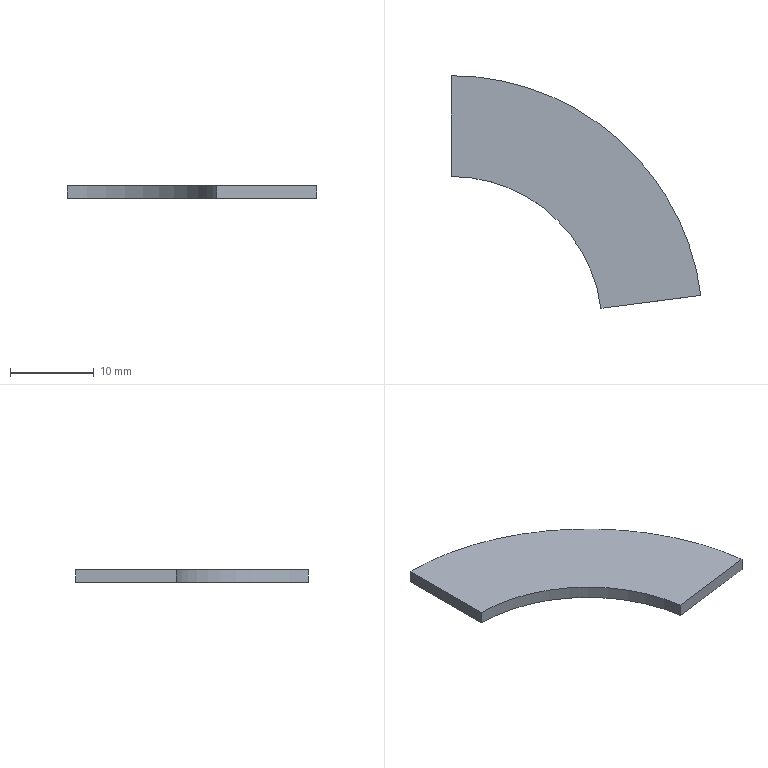Part | STEP file | FHD-021-012-D side door A-D | 1 solid | 6 faces | box 29.753 x 27.697 x 1.5 mm | volume 623.148 mm3 | plane 4 | cylinder 2 | commonest cylinder face diameters 36 x1 60 x1
STEP:
#1=CARTESIAN_POINT('',(0.,0.,0.));
#2=DIRECTION('',(0.,0.,1.));
#3=DIRECTION('',(1.,0.,0.));
#4=AXIS2_PLACEMENT_3D('',#1,#2,#3);
#5=CARTESIAN_POINT('',(1852.179,1263.266,-1.5));
#6=VERTEX_POINT('',#5);
#7=CARTESIAN_POINT('',(1864.08,1264.802,-1.5));
#8=VERTEX_POINT('',#7);
#9=CARTESIAN_POINT('',(1852.179,1263.266,-1.5));
#10=DIRECTION('',(0.9918,0.128,0.));
#11=VECTOR('',#10,1.);
#12=LINE('',#9,#11);
#13=CARTESIAN_POINT('',(1834.327,1260.963,-1.5));
#14=DIRECTION('',(0.,0.,1.));
#15=DIRECTION('',(1.,0.,0.));
#16=AXIS2_PLACEMENT_3D('',#13,#14,#15);
#17=PLANE('',#16);
#18=CARTESIAN_POINT('',(17.852,2.303));
#19=DIRECTION('',(0.9918,0.128));
#20=VECTOR('',#19,1.);
#21=LINE('',#18,#20);
#22=(GEOMETRIC_REPRESENTATION_CONTEXT(2)PARAMETRIC_REPRESENTATION_CONTEXT()REPRESENTATION_CONTEXT('',''));
#23=DEFINITIONAL_REPRESENTATION('',(#21),#22);
#24=PCURVE('',#17,#23);
#25=CARTESIAN_POINT('',(1852.179,1263.266,-1.5));
#26=DIRECTION('',(0.128,-0.9918,0.));
#27=DIRECTION('',(0.9918,0.128,0.));
#28=AXIS2_PLACEMENT_3D('',#25,#26,#27);
#29=PLANE('',#28);
#30=CARTESIAN_POINT('',(0.,0.));
#31=DIRECTION('',(1.,0.));
#32=VECTOR('',#31,1.);
#33=LINE('',#30,#32);
#34=(GEOMETRIC_REPRESENTATION_CONTEXT(2)PARAMETRIC_REPRESENTATION_CONTEXT()REPRESENTATION_CONTEXT('',''));
#35=DEFINITIONAL_REPRESENTATION('',(#33),#34);
#36=PCURVE('',#29,#35);
#37=SURFACE_CURVE('',#12,(#24,#36),.PCURVE_S1.);
#38=EDGE_CURVE('',#6,#8,#37,.T.);
#39=ORIENTED_EDGE('',*,*,#38,.F.);
#40=CARTESIAN_POINT('',(1834.327,1278.963,-1.5));
#41=VERTEX_POINT('',#40);
#42=CARTESIAN_POINT('',(1834.327,1260.963,-1.5));
#43=DIRECTION('',(0.,0.,-1.));
#44=DIRECTION('',(1.,0.,0.));
#45=AXIS2_PLACEMENT_3D('',#42,#43,#44);
#46=CIRCLE('',#45,18.);
#47=CARTESIAN_POINT('',(18.,0.));
#48=CARTESIAN_POINT('',(18.,-31.177));
#49=CARTESIAN_POINT('',(-9.,-15.588));
#50=CARTESIAN_POINT('',(-36.,0.));
#51=CARTESIAN_POINT('',(-9.,15.588));
#52=CARTESIAN_POINT('',(18.,31.177));
#53=CARTESIAN_POINT('',(18.,0.));
#54=(BOUNDED_CURVE()B_SPLINE_CURVE(2,(#47,#48,#49,#50,#51,#52,#53),.UNSPECIFIED.,.T.,.F.)B_SPLINE_CURVE_WITH_KNOTS((1,2,2,2,2,1),(-2.094,0.,2.094,4.189,6.283,8.378),.UNSPECIFIED.)CURVE()GEOMETRIC_REPRESENTATION_ITEM()RATIONAL_B_SPLINE_CURVE((1.,0.5,1.,0.5,1.,0.5,1.))REPRESENTATION_ITEM(''));
#55=(GEOMETRIC_REPRESENTATION_CONTEXT(2)PARAMETRIC_REPRESENTATION_CONTEXT()REPRESENTATION_CONTEXT('',''));
#56=DEFINITIONAL_REPRESENTATION('',(#54),#55);
#57=PCURVE('',#17,#56);
#58=CARTESIAN_POINT('',(1834.327,1260.963,-1.5));
#59=DIRECTION('',(0.,0.,1.));
#60=DIRECTION('',(1.,0.,0.));
#61=AXIS2_PLACEMENT_3D('',#58,#59,#60);
#62=CYLINDRICAL_SURFACE('',#61,18.);
#63=CARTESIAN_POINT('',(6.283,0.));
#64=DIRECTION('',(-1.,0.));
#65=VECTOR('',#64,1.);
#66=LINE('',#63,#65);
#67=(GEOMETRIC_REPRESENTATION_CONTEXT(2)PARAMETRIC_REPRESENTATION_CONTEXT()REPRESENTATION_CONTEXT('',''));
#68=DEFINITIONAL_REPRESENTATION('',(#66),#67);
#69=PCURVE('',#62,#68);
#70=SURFACE_CURVE('',#46,(#57,#69),.PCURVE_S1.);
#71=EDGE_CURVE('',#41,#6,#70,.T.);
#72=ORIENTED_EDGE('',*,*,#71,.F.);
#73=CARTESIAN_POINT('',(1834.327,1290.963,-1.5));
#74=VERTEX_POINT('',#73);
#75=CARTESIAN_POINT('',(1834.327,1260.963,-1.5));
#76=DIRECTION('',(0.,-1.,0.));
#77=VECTOR('',#76,1.);
#78=LINE('',#75,#77);
#79=CARTESIAN_POINT('',(0.,0.));
#80=DIRECTION('',(0.,-1.));
#81=VECTOR('',#80,1.);
#82=LINE('',#79,#81);
#83=(GEOMETRIC_REPRESENTATION_CONTEXT(2)PARAMETRIC_REPRESENTATION_CONTEXT()REPRESENTATION_CONTEXT('',''));
#84=DEFINITIONAL_REPRESENTATION('',(#82),#83);
#85=PCURVE('',#17,#84);
#86=CARTESIAN_POINT('',(1834.327,1290.963,-1.5));
#87=DIRECTION('',(-1.,0.,0.));
#88=DIRECTION('',(0.,0.,1.));
#89=AXIS2_PLACEMENT_3D('',#86,#87,#88);
#90=PLANE('',#89);
#91=CARTESIAN_POINT('',(0.,-30.));
#92=DIRECTION('',(0.,-1.));
#93=VECTOR('',#92,1.);
#94=LINE('',#91,#93);
#95=(GEOMETRIC_REPRESENTATION_CONTEXT(2)PARAMETRIC_REPRESENTATION_CONTEXT()REPRESENTATION_CONTEXT('',''));
#96=DEFINITIONAL_REPRESENTATION('',(#94),#95);
#97=PCURVE('',#90,#96);
#98=SURFACE_CURVE('',#78,(#85,#97),.PCURVE_S1.);
#99=EDGE_CURVE('',#74,#41,#98,.T.);
#100=ORIENTED_EDGE('',*,*,#99,.F.);
#101=CARTESIAN_POINT('',(1834.327,1260.963,-1.5));
#102=DIRECTION('',(0.,0.,1.));
#103=DIRECTION('',(1.,0.,0.));
#104=AXIS2_PLACEMENT_3D('',#101,#102,#103);
#105=CIRCLE('',#104,30.);
#106=CARTESIAN_POINT('',(0.,0.));
#107=DIRECTION('',(1.,0.));
#108=AXIS2_PLACEMENT_2D('',#106,#107);
#109=CIRCLE('',#108,30.);
#110=(GEOMETRIC_REPRESENTATION_CONTEXT(2)PARAMETRIC_REPRESENTATION_CONTEXT()REPRESENTATION_CONTEXT('',''));
#111=DEFINITIONAL_REPRESENTATION('',(#109),#110);
#112=PCURVE('',#17,#111);
#113=CARTESIAN_POINT('',(1834.327,1260.963,-1.5));
#114=DIRECTION('',(0.,0.,1.));
#115=DIRECTION('',(1.,0.,0.));
#116=AXIS2_PLACEMENT_3D('',#113,#114,#115);
#117=CYLINDRICAL_SURFACE('',#116,30.);
#118=CARTESIAN_POINT('',(0.,0.));
#119=DIRECTION('',(1.,0.));
#120=VECTOR('',#119,1.);
#121=LINE('',#118,#120);
#122=(GEOMETRIC_REPRESENTATION_CONTEXT(2)PARAMETRIC_REPRESENTATION_CONTEXT()REPRESENTATION_CONTEXT('',''));
#123=DEFINITIONAL_REPRESENTATION('',(#121),#122);
#124=PCURVE('',#117,#123);
#125=SURFACE_CURVE('',#105,(#112,#124),.PCURVE_S1.);
#126=EDGE_CURVE('',#8,#74,#125,.T.);
#127=ORIENTED_EDGE('',*,*,#126,.F.);
#128=EDGE_LOOP('',(#39,#72,#100,#127));
#129=FACE_BOUND('',#128,.T.);
#130=ADVANCED_FACE('',(#129),#17,.F.);
#131=ORIENTED_EDGE('',*,*,#126,.T.);
#132=CARTESIAN_POINT('',(1834.327,1290.963,0.));
#133=VERTEX_POINT('',#132);
#134=CARTESIAN_POINT('',(1834.327,1290.963,-1.5));
#135=DIRECTION('',(0.,0.,1.));
#136=VECTOR('',#135,1.);
#137=LINE('',#134,#136);
#138=CARTESIAN_POINT('',(1.571,0.));
#139=DIRECTION('',(0.,1.));
#140=VECTOR('',#139,1.);
#141=LINE('',#138,#140);
#142=(GEOMETRIC_REPRESENTATION_CONTEXT(2)PARAMETRIC_REPRESENTATION_CONTEXT()REPRESENTATION_CONTEXT('',''));
#143=DEFINITIONAL_REPRESENTATION('',(#141),#142);
#144=PCURVE('',#117,#143);
#145=CARTESIAN_POINT('',(0.,0.));
#146=DIRECTION('',(1.,0.));
#147=VECTOR('',#146,1.);
#148=LINE('',#145,#147);
#149=(GEOMETRIC_REPRESENTATION_CONTEXT(2)PARAMETRIC_REPRESENTATION_CONTEXT()REPRESENTATION_CONTEXT('',''));
#150=DEFINITIONAL_REPRESENTATION('',(#148),#149);
#151=PCURVE('',#90,#150);
#152=SURFACE_CURVE('',#137,(#144,#151),.PCURVE_S1.);
#153=EDGE_CURVE('',#74,#133,#152,.T.);
#154=ORIENTED_EDGE('',*,*,#153,.T.);
#155=CARTESIAN_POINT('',(1864.08,1264.802,0.));
#156=VERTEX_POINT('',#155);
#157=CARTESIAN_POINT('',(1834.327,1260.963,0.));
#158=DIRECTION('',(0.,0.,-1.));
#159=DIRECTION('',(1.,0.,0.));
#160=AXIS2_PLACEMENT_3D('',#157,#158,#159);
#161=CIRCLE('',#160,30.);
#162=CARTESIAN_POINT('',(6.283,1.5));
#163=DIRECTION('',(-1.,0.));
#164=VECTOR('',#163,1.);
#165=LINE('',#162,#164);
#166=(GEOMETRIC_REPRESENTATION_CONTEXT(2)PARAMETRIC_REPRESENTATION_CONTEXT()REPRESENTATION_CONTEXT('',''));
#167=DEFINITIONAL_REPRESENTATION('',(#165),#166);
#168=PCURVE('',#117,#167);
#169=CARTESIAN_POINT('',(1834.327,1260.963,0.));
#170=DIRECTION('',(0.,0.,1.));
#171=DIRECTION('',(1.,0.,0.));
#172=AXIS2_PLACEMENT_3D('',#169,#170,#171);
#173=PLANE('',#172);
#174=CARTESIAN_POINT('',(30.,0.));
#175=CARTESIAN_POINT('',(30.,-51.962));
#176=CARTESIAN_POINT('',(-15.,-25.981));
#177=CARTESIAN_POINT('',(-60.,0.));
#178=CARTESIAN_POINT('',(-15.,25.981));
#179=CARTESIAN_POINT('',(30.,51.962));
#180=CARTESIAN_POINT('',(30.,0.));
#181=(BOUNDED_CURVE()B_SPLINE_CURVE(2,(#174,#175,#176,#177,#178,#179,#180),.UNSPECIFIED.,.T.,.F.)B_SPLINE_CURVE_WITH_KNOTS((1,2,2,2,2,1),(-2.094,0.,2.094,4.189,6.283,8.378),.UNSPECIFIED.)CURVE()GEOMETRIC_REPRESENTATION_ITEM()RATIONAL_B_SPLINE_CURVE((1.,0.5,1.,0.5,1.,0.5,1.))REPRESENTATION_ITEM(''));
#182=(GEOMETRIC_REPRESENTATION_CONTEXT(2)PARAMETRIC_REPRESENTATION_CONTEXT()REPRESENTATION_CONTEXT('',''));
#183=DEFINITIONAL_REPRESENTATION('',(#181),#182);
#184=PCURVE('',#173,#183);
#185=SURFACE_CURVE('',#161,(#168,#184),.PCURVE_S1.);
#186=EDGE_CURVE('',#133,#156,#185,.T.);
#187=ORIENTED_EDGE('',*,*,#186,.T.);
#188=CARTESIAN_POINT('',(1864.08,1264.802,-1.5));
#189=DIRECTION('',(0.,0.,-1.));
#190=VECTOR('',#189,1.);
#191=LINE('',#188,#190);
#192=CARTESIAN_POINT('',(0.1283,0.));
#193=DIRECTION('',(0.,-1.));
#194=VECTOR('',#193,1.);
#195=LINE('',#192,#194);
#196=(GEOMETRIC_REPRESENTATION_CONTEXT(2)PARAMETRIC_REPRESENTATION_CONTEXT()REPRESENTATION_CONTEXT('',''));
#197=DEFINITIONAL_REPRESENTATION('',(#195),#196);
#198=PCURVE('',#117,#197);
#199=CARTESIAN_POINT('',(12.,0.));
#200=DIRECTION('',(0.,-1.));
#201=VECTOR('',#200,1.);
#202=LINE('',#199,#201);
#203=(GEOMETRIC_REPRESENTATION_CONTEXT(2)PARAMETRIC_REPRESENTATION_CONTEXT()REPRESENTATION_CONTEXT('',''));
#204=DEFINITIONAL_REPRESENTATION('',(#202),#203);
#205=PCURVE('',#29,#204);
#206=SURFACE_CURVE('',#191,(#198,#205),.PCURVE_S1.);
#207=EDGE_CURVE('',#156,#8,#206,.T.);
#208=ORIENTED_EDGE('',*,*,#207,.T.);
#209=EDGE_LOOP('',(#131,#154,#187,#208));
#210=FACE_BOUND('',#209,.T.);
#211=ADVANCED_FACE('',(#210),#117,.T.);
#212=ORIENTED_EDGE('',*,*,#38,.T.);
#213=ORIENTED_EDGE('',*,*,#207,.F.);
#214=CARTESIAN_POINT('',(1852.179,1263.266,0.));
#215=VERTEX_POINT('',#214);
#216=CARTESIAN_POINT('',(1852.179,1263.266,0.));
#217=DIRECTION('',(-0.9918,-0.128,0.));
#218=VECTOR('',#217,1.);
#219=LINE('',#216,#218);
#220=CARTESIAN_POINT('',(0.,1.5));
#221=DIRECTION('',(-1.,0.));
#222=VECTOR('',#221,1.);
#223=LINE('',#220,#222);
#224=(GEOMETRIC_REPRESENTATION_CONTEXT(2)PARAMETRIC_REPRESENTATION_CONTEXT()REPRESENTATION_CONTEXT('',''));
#225=DEFINITIONAL_REPRESENTATION('',(#223),#224);
#226=PCURVE('',#29,#225);
#227=CARTESIAN_POINT('',(17.852,2.303));
#228=DIRECTION('',(-0.9918,-0.128));
#229=VECTOR('',#228,1.);
#230=LINE('',#227,#229);
#231=(GEOMETRIC_REPRESENTATION_CONTEXT(2)PARAMETRIC_REPRESENTATION_CONTEXT()REPRESENTATION_CONTEXT('',''));
#232=DEFINITIONAL_REPRESENTATION('',(#230),#231);
#233=PCURVE('',#173,#232);
#234=SURFACE_CURVE('',#219,(#226,#233),.PCURVE_S1.);
#235=EDGE_CURVE('',#156,#215,#234,.T.);
#236=ORIENTED_EDGE('',*,*,#235,.T.);
#237=CARTESIAN_POINT('',(1852.179,1263.266,-1.5));
#238=DIRECTION('',(0.,0.,-1.));
#239=VECTOR('',#238,1.);
#240=LINE('',#237,#239);
#241=CARTESIAN_POINT('',(0.,0.));
#242=DIRECTION('',(0.,-1.));
#243=VECTOR('',#242,1.);
#244=LINE('',#241,#243);
#245=(GEOMETRIC_REPRESENTATION_CONTEXT(2)PARAMETRIC_REPRESENTATION_CONTEXT()REPRESENTATION_CONTEXT('',''));
#246=DEFINITIONAL_REPRESENTATION('',(#244),#245);
#247=PCURVE('',#29,#246);
#248=CARTESIAN_POINT('',(0.1283,0.));
#249=DIRECTION('',(0.,-1.));
#250=VECTOR('',#249,1.);
#251=LINE('',#248,#250);
#252=(GEOMETRIC_REPRESENTATION_CONTEXT(2)PARAMETRIC_REPRESENTATION_CONTEXT()REPRESENTATION_CONTEXT('',''));
#253=DEFINITIONAL_REPRESENTATION('',(#251),#252);
#254=PCURVE('',#62,#253);
#255=SURFACE_CURVE('',#240,(#247,#254),.PCURVE_S1.);
#256=EDGE_CURVE('',#215,#6,#255,.T.);
#257=ORIENTED_EDGE('',*,*,#256,.T.);
#258=EDGE_LOOP('',(#212,#213,#236,#257));
#259=FACE_BOUND('',#258,.T.);
#260=ADVANCED_FACE('',(#259),#29,.T.);
#261=CARTESIAN_POINT('',(1834.327,1278.963,0.));
#262=VERTEX_POINT('',#261);
#263=CARTESIAN_POINT('',(1834.327,1260.963,0.));
#264=DIRECTION('',(0.,0.,-1.));
#265=DIRECTION('',(1.,0.,0.));
#266=AXIS2_PLACEMENT_3D('',#263,#264,#265);
#267=CIRCLE('',#266,18.);
#268=CARTESIAN_POINT('',(6.283,1.5));
#269=DIRECTION('',(-1.,0.));
#270=VECTOR('',#269,1.);
#271=LINE('',#268,#270);
#272=(GEOMETRIC_REPRESENTATION_CONTEXT(2)PARAMETRIC_REPRESENTATION_CONTEXT()REPRESENTATION_CONTEXT('',''));
#273=DEFINITIONAL_REPRESENTATION('',(#271),#272);
#274=PCURVE('',#62,#273);
#275=CARTESIAN_POINT('',(18.,0.));
#276=CARTESIAN_POINT('',(18.,-31.177));
#277=CARTESIAN_POINT('',(-9.,-15.588));
#278=CARTESIAN_POINT('',(-36.,0.));
#279=CARTESIAN_POINT('',(-9.,15.588));
#280=CARTESIAN_POINT('',(18.,31.177));
#281=CARTESIAN_POINT('',(18.,0.));
#282=(BOUNDED_CURVE()B_SPLINE_CURVE(2,(#275,#276,#277,#278,#279,#280,#281),.UNSPECIFIED.,.T.,.F.)B_SPLINE_CURVE_WITH_KNOTS((1,2,2,2,2,1),(-2.094,0.,2.094,4.189,6.283,8.378),.UNSPECIFIED.)CURVE()GEOMETRIC_REPRESENTATION_ITEM()RATIONAL_B_SPLINE_CURVE((1.,0.5,1.,0.5,1.,0.5,1.))REPRESENTATION_ITEM(''));
#283=(GEOMETRIC_REPRESENTATION_CONTEXT(2)PARAMETRIC_REPRESENTATION_CONTEXT()REPRESENTATION_CONTEXT('',''));
#284=DEFINITIONAL_REPRESENTATION('',(#282),#283);
#285=PCURVE('',#173,#284);
#286=SURFACE_CURVE('',#267,(#274,#285),.PCURVE_S1.);
#287=EDGE_CURVE('',#262,#215,#286,.T.);
#288=ORIENTED_EDGE('',*,*,#287,.T.);
#289=ORIENTED_EDGE('',*,*,#256,.T.);
#290=ORIENTED_EDGE('',*,*,#71,.F.);
#291=CARTESIAN_POINT('',(1834.327,1278.963,-1.5));
#292=DIRECTION('',(0.,0.,1.));
#293=VECTOR('',#292,1.);
#294=LINE('',#291,#293);
#295=CARTESIAN_POINT('',(1.571,0.));
#296=DIRECTION('',(0.,1.));
#297=VECTOR('',#296,1.);
#298=LINE('',#295,#297);
#299=(GEOMETRIC_REPRESENTATION_CONTEXT(2)PARAMETRIC_REPRESENTATION_CONTEXT()REPRESENTATION_CONTEXT('',''));
#300=DEFINITIONAL_REPRESENTATION('',(#298),#299);
#301=PCURVE('',#62,#300);
#302=CARTESIAN_POINT('',(0.,-12.));
#303=DIRECTION('',(1.,0.));
#304=VECTOR('',#303,1.);
#305=LINE('',#302,#304);
#306=(GEOMETRIC_REPRESENTATION_CONTEXT(2)PARAMETRIC_REPRESENTATION_CONTEXT()REPRESENTATION_CONTEXT('',''));
#307=DEFINITIONAL_REPRESENTATION('',(#305),#306);
#308=PCURVE('',#90,#307);
#309=SURFACE_CURVE('',#294,(#301,#308),.PCURVE_S1.);
#310=EDGE_CURVE('',#41,#262,#309,.T.);
#311=ORIENTED_EDGE('',*,*,#310,.T.);
#312=EDGE_LOOP('',(#288,#289,#290,#311));
#313=FACE_BOUND('',#312,.F.);
#314=ADVANCED_FACE('',(#313),#62,.F.);
#315=ORIENTED_EDGE('',*,*,#99,.T.);
#316=ORIENTED_EDGE('',*,*,#310,.T.);
#317=CARTESIAN_POINT('',(1834.327,1290.963,0.));
#318=DIRECTION('',(0.,1.,0.));
#319=VECTOR('',#318,1.);
#320=LINE('',#317,#319);
#321=CARTESIAN_POINT('',(1.5,0.));
#322=DIRECTION('',(0.,1.));
#323=VECTOR('',#322,1.);
#324=LINE('',#321,#323);
#325=(GEOMETRIC_REPRESENTATION_CONTEXT(2)PARAMETRIC_REPRESENTATION_CONTEXT()REPRESENTATION_CONTEXT('',''));
#326=DEFINITIONAL_REPRESENTATION('',(#324),#325);
#327=PCURVE('',#90,#326);
#328=CARTESIAN_POINT('',(0.,30.));
#329=DIRECTION('',(0.,1.));
#330=VECTOR('',#329,1.);
#331=LINE('',#328,#330);
#332=(GEOMETRIC_REPRESENTATION_CONTEXT(2)PARAMETRIC_REPRESENTATION_CONTEXT()REPRESENTATION_CONTEXT('',''));
#333=DEFINITIONAL_REPRESENTATION('',(#331),#332);
#334=PCURVE('',#173,#333);
#335=SURFACE_CURVE('',#320,(#327,#334),.PCURVE_S1.);
#336=EDGE_CURVE('',#262,#133,#335,.T.);
#337=ORIENTED_EDGE('',*,*,#336,.T.);
#338=ORIENTED_EDGE('',*,*,#153,.F.);
#339=EDGE_LOOP('',(#315,#316,#337,#338));
#340=FACE_BOUND('',#339,.T.);
#341=ADVANCED_FACE('',(#340),#90,.T.);
#342=ORIENTED_EDGE('',*,*,#287,.T.);
#343=ORIENTED_EDGE('',*,*,#235,.F.);
#344=ORIENTED_EDGE('',*,*,#186,.F.);
#345=ORIENTED_EDGE('',*,*,#336,.F.);
#346=EDGE_LOOP('',(#342,#343,#344,#345));
#347=FACE_BOUND('',#346,.T.);
#348=ADVANCED_FACE('',(#347),#173,.T.);
#349=CLOSED_SHELL('',(#130,#211,#260,#314,#341,#348));
#350=MANIFOLD_SOLID_BREP('',#349);
#351=(LENGTH_UNIT()NAMED_UNIT(*)SI_UNIT(.MILLI.,.METRE.));
#352=UNCERTAINTY_MEASURE_WITH_UNIT(LENGTH_MEASURE(0.0000001),#351,'','');
#353=(NAMED_UNIT(*)PLANE_ANGLE_UNIT()SI_UNIT($,.RADIAN.));
#354=(NAMED_UNIT(*)SI_UNIT($,.STERADIAN.)SOLID_ANGLE_UNIT());
#355=(GEOMETRIC_REPRESENTATION_CONTEXT(3)GLOBAL_UNCERTAINTY_ASSIGNED_CONTEXT((#352))GLOBAL_UNIT_ASSIGNED_CONTEXT((#351,#353,#354))REPRESENTATION_CONTEXT('',''));
#356=ADVANCED_BREP_SHAPE_REPRESENTATION('',(#4,#350),#355);